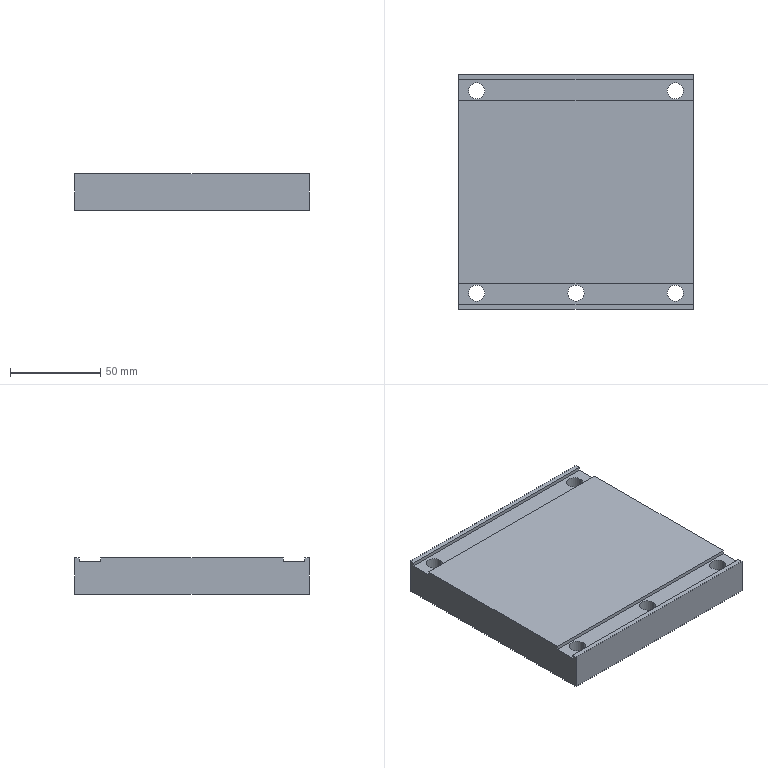Part | STEP file | Head fixing plate | 1 solid | 46 faces | box 130 x 130 x 20 mm | volume 311924 mm3 | cylinder 23 | plane 23 | commonest cylinder face diameters 9 x10 15 x10 3 x3
STEP:
#1=CARTESIAN_POINT('',(62.5,56.,-1.));
#2=VERTEX_POINT('',#1);
#3=CARTESIAN_POINT('',(47.5,56.,-1.));
#4=VERTEX_POINT('',#3);
#5=CARTESIAN_POINT('',(55.,56.,-1.));
#6=DIRECTION('',(0.,0.,-1.));
#7=DIRECTION('',(-1.,0.,0.));
#8=AXIS2_PLACEMENT_3D('',#5,#6,#7);
#9=CIRCLE('',#8,7.5);
#10=EDGE_CURVE('',#2,#4,#9,.T.);
#11=ORIENTED_EDGE('',*,*,#10,.F.);
#12=CARTESIAN_POINT('',(62.5,56.,-10.));
#13=VERTEX_POINT('',#12);
#14=CARTESIAN_POINT('',(62.5,56.,-10.));
#15=DIRECTION('',(0.,0.,-1.));
#16=VECTOR('',#15,1000.);
#17=LINE('',#14,#16);
#18=EDGE_CURVE('',#2,#13,#17,.T.);
#19=ORIENTED_EDGE('',*,*,#18,.T.);
#20=CARTESIAN_POINT('',(47.5,56.,-10.));
#21=VERTEX_POINT('',#20);
#22=CARTESIAN_POINT('',(55.,56.,-10.));
#23=DIRECTION('',(0.,0.,-1.));
#24=DIRECTION('',(-1.,0.,0.));
#25=AXIS2_PLACEMENT_3D('',#22,#23,#24);
#26=CIRCLE('',#25,7.5);
#27=EDGE_CURVE('',#13,#21,#26,.T.);
#28=ORIENTED_EDGE('',*,*,#27,.T.);
#29=CARTESIAN_POINT('',(47.5,56.,-10.));
#30=DIRECTION('',(0.,0.,-1.));
#31=VECTOR('',#30,1000.);
#32=LINE('',#29,#31);
#33=EDGE_CURVE('',#4,#21,#32,.T.);
#34=ORIENTED_EDGE('',*,*,#33,.F.);
#35=EDGE_LOOP('',(#11,#19,#28,#34));
#36=FACE_OUTER_BOUND('',#35,.T.);
#37=CARTESIAN_POINT('',(55.,56.,-10.));
#38=DIRECTION('',(0.,0.,-1.));
#39=DIRECTION('',(-1.,0.,0.));
#40=AXIS2_PLACEMENT_3D('',#37,#38,#39);
#41=CYLINDRICAL_SURFACE('',#40,7.5);
#42=ADVANCED_FACE('',(#36),#41,.F.);
#43=CARTESIAN_POINT('',(50.5,56.,8.));
#44=VERTEX_POINT('',#43);
#45=CARTESIAN_POINT('',(59.5,56.,8.));
#46=VERTEX_POINT('',#45);
#47=CARTESIAN_POINT('',(55.,56.,8.));
#48=DIRECTION('',(0.,0.,1.));
#49=DIRECTION('',(1.,0.,0.));
#50=AXIS2_PLACEMENT_3D('',#47,#48,#49);
#51=CIRCLE('',#50,4.5);
#52=EDGE_CURVE('',#44,#46,#51,.T.);
#53=ORIENTED_EDGE('',*,*,#52,.T.);
#54=CARTESIAN_POINT('',(59.5,56.,-1.));
#55=VERTEX_POINT('',#54);
#56=CARTESIAN_POINT('',(59.5,56.,-10.));
#57=DIRECTION('',(0.,0.,-1.));
#58=VECTOR('',#57,1000.);
#59=LINE('',#56,#58);
#60=EDGE_CURVE('',#46,#55,#59,.T.);
#61=ORIENTED_EDGE('',*,*,#60,.T.);
#62=CARTESIAN_POINT('',(50.5,56.,-1.));
#63=VERTEX_POINT('',#62);
#64=CARTESIAN_POINT('',(55.,56.,-1.));
#65=DIRECTION('',(0.,0.,-1.));
#66=DIRECTION('',(-1.,0.,0.));
#67=AXIS2_PLACEMENT_3D('',#64,#65,#66);
#68=CIRCLE('',#67,4.5);
#69=EDGE_CURVE('',#55,#63,#68,.T.);
#70=ORIENTED_EDGE('',*,*,#69,.T.);
#71=CARTESIAN_POINT('',(50.5,56.,-10.));
#72=DIRECTION('',(0.,0.,-1.));
#73=VECTOR('',#72,1000.);
#74=LINE('',#71,#73);
#75=EDGE_CURVE('',#44,#63,#74,.T.);
#76=ORIENTED_EDGE('',*,*,#75,.F.);
#77=EDGE_LOOP('',(#53,#61,#70,#76));
#78=FACE_OUTER_BOUND('',#77,.T.);
#79=CARTESIAN_POINT('',(55.,56.,-10.));
#80=DIRECTION('',(0.,0.,-1.));
#81=DIRECTION('',(-1.,0.,0.));
#82=AXIS2_PLACEMENT_3D('',#79,#80,#81);
#83=CYLINDRICAL_SURFACE('',#82,4.5);
#84=ADVANCED_FACE('',(#78),#83,.F.);
#85=CARTESIAN_POINT('',(-47.5,56.,-1.));
#86=VERTEX_POINT('',#85);
#87=CARTESIAN_POINT('',(-62.5,56.,-1.));
#88=VERTEX_POINT('',#87);
#89=CARTESIAN_POINT('',(-55.,56.,-1.));
#90=DIRECTION('',(0.,0.,-1.));
#91=DIRECTION('',(-1.,0.,0.));
#92=AXIS2_PLACEMENT_3D('',#89,#90,#91);
#93=CIRCLE('',#92,7.5);
#94=EDGE_CURVE('',#86,#88,#93,.T.);
#95=ORIENTED_EDGE('',*,*,#94,.F.);
#96=CARTESIAN_POINT('',(-47.5,56.,-10.));
#97=VERTEX_POINT('',#96);
#98=CARTESIAN_POINT('',(-47.5,56.,-10.));
#99=DIRECTION('',(0.,0.,-1.));
#100=VECTOR('',#99,1000.);
#101=LINE('',#98,#100);
#102=EDGE_CURVE('',#86,#97,#101,.T.);
#103=ORIENTED_EDGE('',*,*,#102,.T.);
#104=CARTESIAN_POINT('',(-62.5,56.,-10.));
#105=VERTEX_POINT('',#104);
#106=CARTESIAN_POINT('',(-55.,56.,-10.));
#107=DIRECTION('',(0.,0.,-1.));
#108=DIRECTION('',(-1.,0.,0.));
#109=AXIS2_PLACEMENT_3D('',#106,#107,#108);
#110=CIRCLE('',#109,7.5);
#111=EDGE_CURVE('',#97,#105,#110,.T.);
#112=ORIENTED_EDGE('',*,*,#111,.T.);
#113=CARTESIAN_POINT('',(-62.5,56.,-10.));
#114=DIRECTION('',(0.,0.,-1.));
#115=VECTOR('',#114,1000.);
#116=LINE('',#113,#115);
#117=EDGE_CURVE('',#88,#105,#116,.T.);
#118=ORIENTED_EDGE('',*,*,#117,.F.);
#119=EDGE_LOOP('',(#95,#103,#112,#118));
#120=FACE_OUTER_BOUND('',#119,.T.);
#121=CARTESIAN_POINT('',(-55.,56.,-10.));
#122=DIRECTION('',(0.,0.,-1.));
#123=DIRECTION('',(-1.,0.,0.));
#124=AXIS2_PLACEMENT_3D('',#121,#122,#123);
#125=CYLINDRICAL_SURFACE('',#124,7.5);
#126=ADVANCED_FACE('',(#120),#125,.F.);
#127=CARTESIAN_POINT('',(-59.5,56.,8.));
#128=VERTEX_POINT('',#127);
#129=CARTESIAN_POINT('',(-50.5,56.,8.));
#130=VERTEX_POINT('',#129);
#131=CARTESIAN_POINT('',(-55.,56.,8.));
#132=DIRECTION('',(0.,0.,1.));
#133=DIRECTION('',(1.,0.,0.));
#134=AXIS2_PLACEMENT_3D('',#131,#132,#133);
#135=CIRCLE('',#134,4.5);
#136=EDGE_CURVE('',#128,#130,#135,.T.);
#137=ORIENTED_EDGE('',*,*,#136,.T.);
#138=CARTESIAN_POINT('',(-50.5,56.,-1.));
#139=VERTEX_POINT('',#138);
#140=CARTESIAN_POINT('',(-50.5,56.,-10.));
#141=DIRECTION('',(0.,0.,-1.));
#142=VECTOR('',#141,1000.);
#143=LINE('',#140,#142);
#144=EDGE_CURVE('',#130,#139,#143,.T.);
#145=ORIENTED_EDGE('',*,*,#144,.T.);
#146=CARTESIAN_POINT('',(-59.5,56.,-1.));
#147=VERTEX_POINT('',#146);
#148=CARTESIAN_POINT('',(-55.,56.,-1.));
#149=DIRECTION('',(0.,0.,-1.));
#150=DIRECTION('',(-1.,0.,0.));
#151=AXIS2_PLACEMENT_3D('',#148,#149,#150);
#152=CIRCLE('',#151,4.5);
#153=EDGE_CURVE('',#139,#147,#152,.T.);
#154=ORIENTED_EDGE('',*,*,#153,.T.);
#155=CARTESIAN_POINT('',(-59.5,56.,-10.));
#156=DIRECTION('',(0.,0.,-1.));
#157=VECTOR('',#156,1000.);
#158=LINE('',#155,#157);
#159=EDGE_CURVE('',#128,#147,#158,.T.);
#160=ORIENTED_EDGE('',*,*,#159,.F.);
#161=EDGE_LOOP('',(#137,#145,#154,#160));
#162=FACE_OUTER_BOUND('',#161,.T.);
#163=CARTESIAN_POINT('',(-55.,56.,-10.));
#164=DIRECTION('',(0.,0.,-1.));
#165=DIRECTION('',(-1.,0.,0.));
#166=AXIS2_PLACEMENT_3D('',#163,#164,#165);
#167=CYLINDRICAL_SURFACE('',#166,4.5);
#168=ADVANCED_FACE('',(#162),#167,.F.);
#169=CARTESIAN_POINT('',(62.5,-56.,-1.));
#170=VERTEX_POINT('',#169);
#171=CARTESIAN_POINT('',(47.5,-56.,-1.));
#172=VERTEX_POINT('',#171);
#173=CARTESIAN_POINT('',(55.,-56.,-1.));
#174=DIRECTION('',(0.,0.,-1.));
#175=DIRECTION('',(-1.,0.,0.));
#176=AXIS2_PLACEMENT_3D('',#173,#174,#175);
#177=CIRCLE('',#176,7.5);
#178=EDGE_CURVE('',#170,#172,#177,.T.);
#179=ORIENTED_EDGE('',*,*,#178,.F.);
#180=CARTESIAN_POINT('',(62.5,-56.,-10.));
#181=VERTEX_POINT('',#180);
#182=CARTESIAN_POINT('',(62.5,-56.,-10.));
#183=DIRECTION('',(0.,0.,-1.));
#184=VECTOR('',#183,1000.);
#185=LINE('',#182,#184);
#186=EDGE_CURVE('',#170,#181,#185,.T.);
#187=ORIENTED_EDGE('',*,*,#186,.T.);
#188=CARTESIAN_POINT('',(47.5,-56.,-10.));
#189=VERTEX_POINT('',#188);
#190=CARTESIAN_POINT('',(55.,-56.,-10.));
#191=DIRECTION('',(0.,0.,-1.));
#192=DIRECTION('',(-1.,0.,0.));
#193=AXIS2_PLACEMENT_3D('',#190,#191,#192);
#194=CIRCLE('',#193,7.5);
#195=EDGE_CURVE('',#181,#189,#194,.T.);
#196=ORIENTED_EDGE('',*,*,#195,.T.);
#197=CARTESIAN_POINT('',(47.5,-56.,-10.));
#198=DIRECTION('',(0.,0.,-1.));
#199=VECTOR('',#198,1000.);
#200=LINE('',#197,#199);
#201=EDGE_CURVE('',#172,#189,#200,.T.);
#202=ORIENTED_EDGE('',*,*,#201,.F.);
#203=EDGE_LOOP('',(#179,#187,#196,#202));
#204=FACE_OUTER_BOUND('',#203,.T.);
#205=CARTESIAN_POINT('',(55.,-56.,-10.));
#206=DIRECTION('',(0.,0.,-1.));
#207=DIRECTION('',(-1.,0.,0.));
#208=AXIS2_PLACEMENT_3D('',#205,#206,#207);
#209=CYLINDRICAL_SURFACE('',#208,7.5);
#210=ADVANCED_FACE('',(#204),#209,.F.);
#211=CARTESIAN_POINT('',(50.5,-56.,8.));
#212=VERTEX_POINT('',#211);
#213=CARTESIAN_POINT('',(59.5,-56.,8.));
#214=VERTEX_POINT('',#213);
#215=CARTESIAN_POINT('',(55.,-56.,8.));
#216=DIRECTION('',(0.,0.,1.));
#217=DIRECTION('',(1.,0.,0.));
#218=AXIS2_PLACEMENT_3D('',#215,#216,#217);
#219=CIRCLE('',#218,4.5);
#220=EDGE_CURVE('',#212,#214,#219,.T.);
#221=ORIENTED_EDGE('',*,*,#220,.T.);
#222=CARTESIAN_POINT('',(59.5,-56.,-1.));
#223=VERTEX_POINT('',#222);
#224=CARTESIAN_POINT('',(59.5,-56.,-10.));
#225=DIRECTION('',(0.,0.,-1.));
#226=VECTOR('',#225,1000.);
#227=LINE('',#224,#226);
#228=EDGE_CURVE('',#214,#223,#227,.T.);
#229=ORIENTED_EDGE('',*,*,#228,.T.);
#230=CARTESIAN_POINT('',(50.5,-56.,-1.));
#231=VERTEX_POINT('',#230);
#232=CARTESIAN_POINT('',(55.,-56.,-1.));
#233=DIRECTION('',(0.,0.,-1.));
#234=DIRECTION('',(-1.,0.,0.));
#235=AXIS2_PLACEMENT_3D('',#232,#233,#234);
#236=CIRCLE('',#235,4.5);
#237=EDGE_CURVE('',#223,#231,#236,.T.);
#238=ORIENTED_EDGE('',*,*,#237,.T.);
#239=CARTESIAN_POINT('',(50.5,-56.,-10.));
#240=DIRECTION('',(0.,0.,-1.));
#241=VECTOR('',#240,1000.);
#242=LINE('',#239,#241);
#243=EDGE_CURVE('',#212,#231,#242,.T.);
#244=ORIENTED_EDGE('',*,*,#243,.F.);
#245=EDGE_LOOP('',(#221,#229,#238,#244));
#246=FACE_OUTER_BOUND('',#245,.T.);
#247=CARTESIAN_POINT('',(55.,-56.,-10.));
#248=DIRECTION('',(0.,0.,-1.));
#249=DIRECTION('',(-1.,0.,0.));
#250=AXIS2_PLACEMENT_3D('',#247,#248,#249);
#251=CYLINDRICAL_SURFACE('',#250,4.5);
#252=ADVANCED_FACE('',(#246),#251,.F.);
#253=CARTESIAN_POINT('',(7.5,-56.,-1.));
#254=VERTEX_POINT('',#253);
#255=CARTESIAN_POINT('',(-7.5,-56.,-1.));
#256=VERTEX_POINT('',#255);
#257=CARTESIAN_POINT('',(0.,-56.,-1.));
#258=DIRECTION('',(0.,0.,-1.));
#259=DIRECTION('',(-1.,0.,0.));
#260=AXIS2_PLACEMENT_3D('',#257,#258,#259);
#261=CIRCLE('',#260,7.5);
#262=EDGE_CURVE('',#254,#256,#261,.T.);
#263=ORIENTED_EDGE('',*,*,#262,.F.);
#264=CARTESIAN_POINT('',(7.5,-56.,-10.));
#265=VERTEX_POINT('',#264);
#266=CARTESIAN_POINT('',(7.5,-56.,-10.));
#267=DIRECTION('',(0.,0.,-1.));
#268=VECTOR('',#267,1000.);
#269=LINE('',#266,#268);
#270=EDGE_CURVE('',#254,#265,#269,.T.);
#271=ORIENTED_EDGE('',*,*,#270,.T.);
#272=CARTESIAN_POINT('',(-7.5,-56.,-10.));
#273=VERTEX_POINT('',#272);
#274=CARTESIAN_POINT('',(0.,-56.,-10.));
#275=DIRECTION('',(0.,0.,-1.));
#276=DIRECTION('',(-1.,0.,0.));
#277=AXIS2_PLACEMENT_3D('',#274,#275,#276);
#278=CIRCLE('',#277,7.5);
#279=EDGE_CURVE('',#265,#273,#278,.T.);
#280=ORIENTED_EDGE('',*,*,#279,.T.);
#281=CARTESIAN_POINT('',(-7.5,-56.,-10.));
#282=DIRECTION('',(0.,0.,-1.));
#283=VECTOR('',#282,1000.);
#284=LINE('',#281,#283);
#285=EDGE_CURVE('',#256,#273,#284,.T.);
#286=ORIENTED_EDGE('',*,*,#285,.F.);
#287=EDGE_LOOP('',(#263,#271,#280,#286));
#288=FACE_OUTER_BOUND('',#287,.T.);
#289=CARTESIAN_POINT('',(0.,-56.,-10.));
#290=DIRECTION('',(0.,0.,-1.));
#291=DIRECTION('',(-1.,0.,0.));
#292=AXIS2_PLACEMENT_3D('',#289,#290,#291);
#293=CYLINDRICAL_SURFACE('',#292,7.5);
#294=ADVANCED_FACE('',(#288),#293,.F.);
#295=CARTESIAN_POINT('',(-4.5,-56.,8.));
#296=VERTEX_POINT('',#295);
#297=CARTESIAN_POINT('',(4.5,-56.,8.));
#298=VERTEX_POINT('',#297);
#299=CARTESIAN_POINT('',(0.,-56.,8.));
#300=DIRECTION('',(0.,0.,1.));
#301=DIRECTION('',(1.,0.,0.));
#302=AXIS2_PLACEMENT_3D('',#299,#300,#301);
#303=CIRCLE('',#302,4.5);
#304=EDGE_CURVE('',#296,#298,#303,.T.);
#305=ORIENTED_EDGE('',*,*,#304,.T.);
#306=CARTESIAN_POINT('',(4.5,-56.,-1.));
#307=VERTEX_POINT('',#306);
#308=CARTESIAN_POINT('',(4.5,-56.,-10.));
#309=DIRECTION('',(0.,0.,-1.));
#310=VECTOR('',#309,1000.);
#311=LINE('',#308,#310);
#312=EDGE_CURVE('',#298,#307,#311,.T.);
#313=ORIENTED_EDGE('',*,*,#312,.T.);
#314=CARTESIAN_POINT('',(-4.5,-56.,-1.));
#315=VERTEX_POINT('',#314);
#316=CARTESIAN_POINT('',(0.,-56.,-1.));
#317=DIRECTION('',(0.,0.,-1.));
#318=DIRECTION('',(-1.,0.,0.));
#319=AXIS2_PLACEMENT_3D('',#316,#317,#318);
#320=CIRCLE('',#319,4.5);
#321=EDGE_CURVE('',#307,#315,#320,.T.);
#322=ORIENTED_EDGE('',*,*,#321,.T.);
#323=CARTESIAN_POINT('',(-4.5,-56.,-10.));
#324=DIRECTION('',(0.,0.,-1.));
#325=VECTOR('',#324,1000.);
#326=LINE('',#323,#325);
#327=EDGE_CURVE('',#296,#315,#326,.T.);
#328=ORIENTED_EDGE('',*,*,#327,.F.);
#329=EDGE_LOOP('',(#305,#313,#322,#328));
#330=FACE_OUTER_BOUND('',#329,.T.);
#331=CARTESIAN_POINT('',(0.,-56.,-10.));
#332=DIRECTION('',(0.,0.,-1.));
#333=DIRECTION('',(-1.,0.,0.));
#334=AXIS2_PLACEMENT_3D('',#331,#332,#333);
#335=CYLINDRICAL_SURFACE('',#334,4.5);
#336=ADVANCED_FACE('',(#330),#335,.F.);
#337=CARTESIAN_POINT('',(-47.5,-56.,-1.));
#338=VERTEX_POINT('',#337);
#339=CARTESIAN_POINT('',(-62.5,-56.,-1.));
#340=VERTEX_POINT('',#339);
#341=CARTESIAN_POINT('',(-55.,-56.,-1.));
#342=DIRECTION('',(0.,0.,-1.));
#343=DIRECTION('',(-1.,0.,0.));
#344=AXIS2_PLACEMENT_3D('',#341,#342,#343);
#345=CIRCLE('',#344,7.5);
#346=EDGE_CURVE('',#338,#340,#345,.T.);
#347=ORIENTED_EDGE('',*,*,#346,.F.);
#348=CARTESIAN_POINT('',(-47.5,-56.,-10.));
#349=VERTEX_POINT('',#348);
#350=CARTESIAN_POINT('',(-47.5,-56.,-10.));
#351=DIRECTION('',(0.,0.,-1.));
#352=VECTOR('',#351,1000.);
#353=LINE('',#350,#352);
#354=EDGE_CURVE('',#338,#349,#353,.T.);
#355=ORIENTED_EDGE('',*,*,#354,.T.);
#356=CARTESIAN_POINT('',(-62.5,-56.,-10.));
#357=VERTEX_POINT('',#356);
#358=CARTESIAN_POINT('',(-55.,-56.,-10.));
#359=DIRECTION('',(0.,0.,-1.));
#360=DIRECTION('',(-1.,0.,0.));
#361=AXIS2_PLACEMENT_3D('',#358,#359,#360);
#362=CIRCLE('',#361,7.5);
#363=EDGE_CURVE('',#349,#357,#362,.T.);
#364=ORIENTED_EDGE('',*,*,#363,.T.);
#365=CARTESIAN_POINT('',(-62.5,-56.,-10.));
#366=DIRECTION('',(0.,0.,-1.));
#367=VECTOR('',#366,1000.);
#368=LINE('',#365,#367);
#369=EDGE_CURVE('',#340,#357,#368,.T.);
#370=ORIENTED_EDGE('',*,*,#369,.F.);
#371=EDGE_LOOP('',(#347,#355,#364,#370));
#372=FACE_OUTER_BOUND('',#371,.T.);
#373=CARTESIAN_POINT('',(-55.,-56.,-10.));
#374=DIRECTION('',(0.,0.,-1.));
#375=DIRECTION('',(-1.,0.,0.));
#376=AXIS2_PLACEMENT_3D('',#373,#374,#375);
#377=CYLINDRICAL_SURFACE('',#376,7.5);
#378=ADVANCED_FACE('',(#372),#377,.F.);
#379=CARTESIAN_POINT('',(-59.5,-56.,8.));
#380=VERTEX_POINT('',#379);
#381=CARTESIAN_POINT('',(-50.5,-56.,8.));
#382=VERTEX_POINT('',#381);
#383=CARTESIAN_POINT('',(-55.,-56.,8.));
#384=DIRECTION('',(0.,0.,1.));
#385=DIRECTION('',(1.,0.,0.));
#386=AXIS2_PLACEMENT_3D('',#383,#384,#385);
#387=CIRCLE('',#386,4.5);
#388=EDGE_CURVE('',#380,#382,#387,.T.);
#389=ORIENTED_EDGE('',*,*,#388,.T.);
#390=CARTESIAN_POINT('',(-50.5,-56.,-1.));
#391=VERTEX_POINT('',#390);
#392=CARTESIAN_POINT('',(-50.5,-56.,-10.));
#393=DIRECTION('',(0.,0.,-1.));
#394=VECTOR('',#393,1000.);
#395=LINE('',#392,#394);
#396=EDGE_CURVE('',#382,#391,#395,.T.);
#397=ORIENTED_EDGE('',*,*,#396,.T.);
#398=CARTESIAN_POINT('',(-59.5,-56.,-1.));
#399=VERTEX_POINT('',#398);
#400=CARTESIAN_POINT('',(-55.,-56.,-1.));
#401=DIRECTION('',(0.,0.,-1.));
#402=DIRECTION('',(-1.,0.,0.));
#403=AXIS2_PLACEMENT_3D('',#400,#401,#402);
#404=CIRCLE('',#403,4.5);
#405=EDGE_CURVE('',#391,#399,#404,.T.);
#406=ORIENTED_EDGE('',*,*,#405,.T.);
#407=CARTESIAN_POINT('',(-59.5,-56.,-10.));
#408=DIRECTION('',(0.,0.,-1.));
#409=VECTOR('',#408,1000.);
#410=LINE('',#407,#409);
#411=EDGE_CURVE('',#380,#399,#410,.T.);
#412=ORIENTED_EDGE('',*,*,#411,.F.);
#413=EDGE_LOOP('',(#389,#397,#406,#412));
#414=FACE_OUTER_BOUND('',#413,.T.);
#415=CARTESIAN_POINT('',(-55.,-56.,-10.));
#416=DIRECTION('',(0.,0.,-1.));
#417=DIRECTION('',(-1.,0.,0.));
#418=AXIS2_PLACEMENT_3D('',#415,#416,#417);
#419=CYLINDRICAL_SURFACE('',#418,4.5);
#420=ADVANCED_FACE('',(#414),#419,.F.);
#421=CARTESIAN_POINT('',(-39.,5.,-8.));
#422=VERTEX_POINT('',#421);
#423=CARTESIAN_POINT('',(-37.5,6.5,-8.));
#424=VERTEX_POINT('',#423);
#425=CARTESIAN_POINT('',(-37.5,5.,-8.));
#426=DIRECTION('',(0.,0.,-1.));
#427=DIRECTION('',(-1.,0.,0.));
#428=AXIS2_PLACEMENT_3D('',#425,#426,#427);
#429=CIRCLE('',#428,1.5);
#430=EDGE_CURVE('',#422,#424,#429,.T.);
#431=ORIENTED_EDGE('',*,*,#430,.F.);
#432=CARTESIAN_POINT('',(-39.,5.,-10.));
#433=VERTEX_POINT('',#432);
#434=CARTESIAN_POINT('',(-39.,5.,-8.));
#435=DIRECTION('',(0.,0.,-1.));
#436=VECTOR('',#435,1000.);
#437=LINE('',#434,#436);
#438=EDGE_CURVE('',#422,#433,#437,.T.);
#439=ORIENTED_EDGE('',*,*,#438,.T.);
#440=CARTESIAN_POINT('',(-37.5,6.5,-10.));
#441=VERTEX_POINT('',#440);
#442=CARTESIAN_POINT('',(-37.5,5.,-10.));
#443=DIRECTION('',(0.,0.,-1.));
#444=DIRECTION('',(-1.,0.,0.));
#445=AXIS2_PLACEMENT_3D('',#442,#443,#444);
#446=CIRCLE('',#445,1.5);
#447=EDGE_CURVE('',#433,#441,#446,.T.);
#448=ORIENTED_EDGE('',*,*,#447,.T.);
#449=CARTESIAN_POINT('',(-37.5,6.5,-8.));
#450=DIRECTION('',(0.,0.,-1.));
#451=VECTOR('',#450,1000.);
#452=LINE('',#449,#451);
#453=EDGE_CURVE('',#424,#441,#452,.T.);
#454=ORIENTED_EDGE('',*,*,#453,.F.);
#455=EDGE_LOOP('',(#431,#439,#448,#454));
#456=FACE_OUTER_BOUND('',#455,.T.);
#457=CARTESIAN_POINT('',(-37.5,5.,-8.));
#458=DIRECTION('',(0.,0.,-1.));
#459=DIRECTION('',(-1.,0.,0.));
#460=AXIS2_PLACEMENT_3D('',#457,#458,#459);
#461=CYLINDRICAL_SURFACE('',#460,1.5);
#462=ADVANCED_FACE('',(#456),#461,.F.);
#463=CARTESIAN_POINT('',(-65.,-62.5,10.));
#464=VERTEX_POINT('',#463);
#465=CARTESIAN_POINT('',(65.,-62.5,10.));
#466=VERTEX_POINT('',#465);
#467=CARTESIAN_POINT('',(-65.,-62.5,10.));
#468=DIRECTION('',(1.,0.,0.));
#469=VECTOR('',#468,1000.);
#470=LINE('',#467,#469);
#471=EDGE_CURVE('',#464,#466,#470,.T.);
#472=ORIENTED_EDGE('',*,*,#471,.F.);
#473=CARTESIAN_POINT('',(-65.,-65.,10.));
#474=VERTEX_POINT('',#473);
#475=CARTESIAN_POINT('',(-65.,65.,10.));
#476=DIRECTION('',(0.,-1.,0.));
#477=VECTOR('',#476,1000.);
#478=LINE('',#475,#477);
#479=EDGE_CURVE('',#464,#474,#478,.T.);
#480=ORIENTED_EDGE('',*,*,#479,.T.);
#481=CARTESIAN_POINT('',(65.,-65.,10.));
#482=VERTEX_POINT('',#481);
#483=CARTESIAN_POINT('',(-65.,-65.,10.));
#484=DIRECTION('',(1.,0.,0.));
#485=VECTOR('',#484,1000.);
#486=LINE('',#483,#485);
#487=EDGE_CURVE('',#474,#482,#486,.T.);
#488=ORIENTED_EDGE('',*,*,#487,.T.);
#489=CARTESIAN_POINT('',(65.,65.,10.));
#490=DIRECTION('',(0.,1.,0.));
#491=VECTOR('',#490,1000.);
#492=LINE('',#489,#491);
#493=EDGE_CURVE('',#482,#466,#492,.T.);
#494=ORIENTED_EDGE('',*,*,#493,.T.);
#495=EDGE_LOOP('',(#472,#480,#488,#494));
#496=FACE_OUTER_BOUND('',#495,.T.);
#497=CARTESIAN_POINT('',(0.,0.,10.));
#498=DIRECTION('',(0.,0.,1.));
#499=DIRECTION('',(1.,0.,0.));
#500=AXIS2_PLACEMENT_3D('',#497,#498,#499);
#501=PLANE('',#500);
#502=ADVANCED_FACE('',(#496),#501,.T.);
#503=CARTESIAN_POINT('',(65.,62.5,10.));
#504=VERTEX_POINT('',#503);
#505=CARTESIAN_POINT('',(-65.,62.5,10.));
#506=VERTEX_POINT('',#505);
#507=CARTESIAN_POINT('',(-65.,62.5,10.));
#508=DIRECTION('',(-1.,0.,0.));
#509=VECTOR('',#508,1000.);
#510=LINE('',#507,#509);
#511=EDGE_CURVE('',#504,#506,#510,.T.);
#512=ORIENTED_EDGE('',*,*,#511,.F.);
#513=CARTESIAN_POINT('',(65.,65.,10.));
#514=VERTEX_POINT('',#513);
#515=CARTESIAN_POINT('',(65.,65.,10.));
#516=DIRECTION('',(0.,1.,0.));
#517=VECTOR('',#516,1000.);
#518=LINE('',#515,#517);
#519=EDGE_CURVE('',#504,#514,#518,.T.);
#520=ORIENTED_EDGE('',*,*,#519,.T.);
#521=CARTESIAN_POINT('',(-65.,65.,10.));
#522=VERTEX_POINT('',#521);
#523=CARTESIAN_POINT('',(-65.,65.,10.));
#524=DIRECTION('',(-1.,0.,0.));
#525=VECTOR('',#524,1000.);
#526=LINE('',#523,#525);
#527=EDGE_CURVE('',#514,#522,#526,.T.);
#528=ORIENTED_EDGE('',*,*,#527,.T.);
#529=CARTESIAN_POINT('',(-65.,65.,10.));
#530=DIRECTION('',(0.,-1.,0.));
#531=VECTOR('',#530,1000.);
#532=LINE('',#529,#531);
#533=EDGE_CURVE('',#522,#506,#532,.T.);
#534=ORIENTED_EDGE('',*,*,#533,.T.);
#535=EDGE_LOOP('',(#512,#520,#528,#534));
#536=FACE_OUTER_BOUND('',#535,.T.);
#537=CARTESIAN_POINT('',(0.,0.,10.));
#538=DIRECTION('',(0.,0.,1.));
#539=DIRECTION('',(1.,0.,0.));
#540=AXIS2_PLACEMENT_3D('',#537,#538,#539);
#541=PLANE('',#540);
#542=ADVANCED_FACE('',(#536),#541,.T.);
#543=CARTESIAN_POINT('',(65.,-62.5,8.));
#544=VERTEX_POINT('',#543);
#545=CARTESIAN_POINT('',(65.,-50.5,8.));
#546=VERTEX_POINT('',#545);
#547=CARTESIAN_POINT('',(65.,-62.5,8.));
#548=DIRECTION('',(0.,1.,0.));
#549=VECTOR('',#548,1000.);
#550=LINE('',#547,#549);
#551=EDGE_CURVE('',#544,#546,#550,.T.);
#552=ORIENTED_EDGE('',*,*,#551,.F.);
#553=CARTESIAN_POINT('',(65.,-62.5,8.));
#554=DIRECTION('',(0.,0.,1.));
#555=VECTOR('',#554,1000.);
#556=LINE('',#553,#555);
#557=EDGE_CURVE('',#544,#466,#556,.T.);
#558=ORIENTED_EDGE('',*,*,#557,.T.);
#559=ORIENTED_EDGE('',*,*,#493,.F.);
#560=CARTESIAN_POINT('',(65.,-65.,-10.));
#561=VERTEX_POINT('',#560);
#562=CARTESIAN_POINT('',(65.,-65.,10.));
#563=DIRECTION('',(0.,0.,-1.));
#564=VECTOR('',#563,1000.);
#565=LINE('',#562,#564);
#566=EDGE_CURVE('',#482,#561,#565,.T.);
#567=ORIENTED_EDGE('',*,*,#566,.T.);
#568=CARTESIAN_POINT('',(65.,65.,-10.));
#569=VERTEX_POINT('',#568);
#570=CARTESIAN_POINT('',(65.,65.,-10.));
#571=DIRECTION('',(0.,1.,0.));
#572=VECTOR('',#571,1000.);
#573=LINE('',#570,#572);
#574=EDGE_CURVE('',#561,#569,#573,.T.);
#575=ORIENTED_EDGE('',*,*,#574,.T.);
#576=CARTESIAN_POINT('',(65.,65.,10.));
#577=DIRECTION('',(0.,0.,-1.));
#578=VECTOR('',#577,1000.);
#579=LINE('',#576,#578);
#580=EDGE_CURVE('',#514,#569,#579,.T.);
#581=ORIENTED_EDGE('',*,*,#580,.F.);
#582=ORIENTED_EDGE('',*,*,#519,.F.);
#583=CARTESIAN_POINT('',(65.,62.5,8.));
#584=VERTEX_POINT('',#583);
#585=CARTESIAN_POINT('',(65.,62.5,8.));
#586=DIRECTION('',(0.,0.,1.));
#587=VECTOR('',#586,1000.);
#588=LINE('',#585,#587);
#589=EDGE_CURVE('',#584,#504,#588,.T.);
#590=ORIENTED_EDGE('',*,*,#589,.F.);
#591=CARTESIAN_POINT('',(65.,50.5,8.));
#592=VERTEX_POINT('',#591);
#593=CARTESIAN_POINT('',(65.,62.5,8.));
#594=DIRECTION('',(0.,1.,0.));
#595=VECTOR('',#594,1000.);
#596=LINE('',#593,#595);
#597=EDGE_CURVE('',#592,#584,#596,.T.);
#598=ORIENTED_EDGE('',*,*,#597,.F.);
#599=CARTESIAN_POINT('',(65.,50.5,10.));
#600=VERTEX_POINT('',#599);
#601=CARTESIAN_POINT('',(65.,50.5,8.));
#602=DIRECTION('',(0.,0.,1.));
#603=VECTOR('',#602,1000.);
#604=LINE('',#601,#603);
#605=EDGE_CURVE('',#592,#600,#604,.T.);
#606=ORIENTED_EDGE('',*,*,#605,.T.);
#607=CARTESIAN_POINT('',(65.,-50.5,10.));
#608=VERTEX_POINT('',#607);
#609=CARTESIAN_POINT('',(65.,65.,10.));
#610=DIRECTION('',(0.,1.,0.));
#611=VECTOR('',#610,1000.);
#612=LINE('',#609,#611);
#613=EDGE_CURVE('',#608,#600,#612,.T.);
#614=ORIENTED_EDGE('',*,*,#613,.F.);
#615=CARTESIAN_POINT('',(65.,-50.5,8.));
#616=DIRECTION('',(0.,0.,1.));
#617=VECTOR('',#616,1000.);
#618=LINE('',#615,#617);
#619=EDGE_CURVE('',#546,#608,#618,.T.);
#620=ORIENTED_EDGE('',*,*,#619,.F.);
#621=EDGE_LOOP('',(#552,#558,#559,#567,#575,#581,#582,#590,#598,#606,#614,#620));
#622=FACE_OUTER_BOUND('',#621,.T.);
#623=CARTESIAN_POINT('',(65.,65.,10.));
#624=DIRECTION('',(-1.,0.,0.));
#625=DIRECTION('',(0.,-1.,0.));
#626=AXIS2_PLACEMENT_3D('',#623,#624,#625);
#627=PLANE('',#626);
#628=ADVANCED_FACE('',(#622),#627,.F.);
#629=CARTESIAN_POINT('',(37.5,65.,-10.));
#630=VERTEX_POINT('',#629);
#631=CARTESIAN_POINT('',(-65.,65.,-10.));
#632=DIRECTION('',(-1.,0.,0.));
#633=VECTOR('',#632,1000.);
#634=LINE('',#631,#633);
#635=EDGE_CURVE('',#569,#630,#634,.T.);
#636=ORIENTED_EDGE('',*,*,#635,.T.);
#637=CARTESIAN_POINT('',(37.5,65.,-8.));
#638=VERTEX_POINT('',#637);
#639=CARTESIAN_POINT('',(37.5,65.,-8.));
#640=DIRECTION('',(0.,0.,-1.));
#641=VECTOR('',#640,1000.);
#642=LINE('',#639,#641);
#643=EDGE_CURVE('',#638,#630,#642,.T.);
#644=ORIENTED_EDGE('',*,*,#643,.F.);
#645=CARTESIAN_POINT('',(-37.5,65.,-8.));
#646=VERTEX_POINT('',#645);
#647=CARTESIAN_POINT('',(37.5,65.,-8.));
#648=DIRECTION('',(1.,0.,0.));
#649=VECTOR('',#648,1000.);
#650=LINE('',#647,#649);
#651=EDGE_CURVE('',#646,#638,#650,.T.);
#652=ORIENTED_EDGE('',*,*,#651,.F.);
#653=CARTESIAN_POINT('',(-37.5,65.,-10.));
#654=VERTEX_POINT('',#653);
#655=CARTESIAN_POINT('',(-37.5,65.,-8.));
#656=DIRECTION('',(0.,0.,-1.));
#657=VECTOR('',#656,1000.);
#658=LINE('',#655,#657);
#659=EDGE_CURVE('',#646,#654,#658,.T.);
#660=ORIENTED_EDGE('',*,*,#659,.T.);
#661=CARTESIAN_POINT('',(-65.,65.,-10.));
#662=VERTEX_POINT('',#661);
#663=CARTESIAN_POINT('',(-65.,65.,-10.));
#664=DIRECTION('',(-1.,0.,0.));
#665=VECTOR('',#664,1000.);
#666=LINE('',#663,#665);
#667=EDGE_CURVE('',#654,#662,#666,.T.);
#668=ORIENTED_EDGE('',*,*,#667,.T.);
#669=CARTESIAN_POINT('',(-65.,65.,10.));
#670=DIRECTION('',(0.,0.,-1.));
#671=VECTOR('',#670,1000.);
#672=LINE('',#669,#671);
#673=EDGE_CURVE('',#522,#662,#672,.T.);
#674=ORIENTED_EDGE('',*,*,#673,.F.);
#675=ORIENTED_EDGE('',*,*,#527,.F.);
#676=ORIENTED_EDGE('',*,*,#580,.T.);
#677=EDGE_LOOP('',(#636,#644,#652,#660,#668,#674,#675,#676));
#678=FACE_OUTER_BOUND('',#677,.T.);
#679=CARTESIAN_POINT('',(-65.,65.,10.));
#680=DIRECTION('',(0.,-1.,0.));
#681=DIRECTION('',(0.,0.,-1.));
#682=AXIS2_PLACEMENT_3D('',#679,#680,#681);
#683=PLANE('',#682);
#684=ADVANCED_FACE('',(#678),#683,.F.);
#685=ORIENTED_EDGE('',*,*,#479,.F.);
#686=CARTESIAN_POINT('',(-65.,-62.5,8.));
#687=VERTEX_POINT('',#686);
#688=CARTESIAN_POINT('',(-65.,-62.5,8.));
#689=DIRECTION('',(0.,0.,1.));
#690=VECTOR('',#689,1000.);
#691=LINE('',#688,#690);
#692=EDGE_CURVE('',#687,#464,#691,.T.);
#693=ORIENTED_EDGE('',*,*,#692,.F.);
#694=CARTESIAN_POINT('',(-65.,-50.5,8.));
#695=VERTEX_POINT('',#694);
#696=CARTESIAN_POINT('',(-65.,-62.5,8.));
#697=DIRECTION('',(0.,-1.,0.));
#698=VECTOR('',#697,1000.);
#699=LINE('',#696,#698);
#700=EDGE_CURVE('',#695,#687,#699,.T.);
#701=ORIENTED_EDGE('',*,*,#700,.F.);
#702=CARTESIAN_POINT('',(-65.,-50.5,10.));
#703=VERTEX_POINT('',#702);
#704=CARTESIAN_POINT('',(-65.,-50.5,8.));
#705=DIRECTION('',(0.,0.,1.));
#706=VECTOR('',#705,1000.);
#707=LINE('',#704,#706);
#708=EDGE_CURVE('',#695,#703,#707,.T.);
#709=ORIENTED_EDGE('',*,*,#708,.T.);
#710=CARTESIAN_POINT('',(-65.,50.5,10.));
#711=VERTEX_POINT('',#710);
#712=CARTESIAN_POINT('',(-65.,65.,10.));
#713=DIRECTION('',(0.,-1.,0.));
#714=VECTOR('',#713,1000.);
#715=LINE('',#712,#714);
#716=EDGE_CURVE('',#711,#703,#715,.T.);
#717=ORIENTED_EDGE('',*,*,#716,.F.);
#718=CARTESIAN_POINT('',(-65.,50.5,8.));
#719=VERTEX_POINT('',#718);
#720=CARTESIAN_POINT('',(-65.,50.5,8.));
#721=DIRECTION('',(0.,0.,1.));
#722=VECTOR('',#721,1000.);
#723=LINE('',#720,#722);
#724=EDGE_CURVE('',#719,#711,#723,.T.);
#725=ORIENTED_EDGE('',*,*,#724,.F.);
#726=CARTESIAN_POINT('',(-65.,62.5,8.));
#727=VERTEX_POINT('',#726);
#728=CARTESIAN_POINT('',(-65.,62.5,8.));
#729=DIRECTION('',(0.,-1.,0.));
#730=VECTOR('',#729,1000.);
#731=LINE('',#728,#730);
#732=EDGE_CURVE('',#727,#719,#731,.T.);
#733=ORIENTED_EDGE('',*,*,#732,.F.);
#734=CARTESIAN_POINT('',(-65.,62.5,8.));
#735=DIRECTION('',(0.,0.,1.));
#736=VECTOR('',#735,1000.);
#737=LINE('',#734,#736);
#738=EDGE_CURVE('',#727,#506,#737,.T.);
#739=ORIENTED_EDGE('',*,*,#738,.T.);
#740=ORIENTED_EDGE('',*,*,#533,.F.);
#741=ORIENTED_EDGE('',*,*,#673,.T.);
#742=CARTESIAN_POINT('',(-65.,-65.,-10.));
#743=VERTEX_POINT('',#742);
#744=CARTESIAN_POINT('',(-65.,65.,-10.));
#745=DIRECTION('',(0.,-1.,0.));
#746=VECTOR('',#745,1000.);
#747=LINE('',#744,#746);
#748=EDGE_CURVE('',#662,#743,#747,.T.);
#749=ORIENTED_EDGE('',*,*,#748,.T.);
#750=CARTESIAN_POINT('',(-65.,-65.,10.));
#751=DIRECTION('',(0.,0.,-1.));
#752=VECTOR('',#751,1000.);
#753=LINE('',#750,#752);
#754=EDGE_CURVE('',#474,#743,#753,.T.);
#755=ORIENTED_EDGE('',*,*,#754,.F.);
#756=EDGE_LOOP('',(#685,#693,#701,#709,#717,#725,#733,#739,#740,#741,#749,#755));
#757=FACE_OUTER_BOUND('',#756,.T.);
#758=CARTESIAN_POINT('',(-65.,65.,10.));
#759=DIRECTION('',(1.,0.,0.));
#760=DIRECTION('',(0.,1.,0.));
#761=AXIS2_PLACEMENT_3D('',#758,#759,#760);
#762=PLANE('',#761);
#763=ADVANCED_FACE('',(#757),#762,.F.);
#764=CARTESIAN_POINT('',(-65.,-65.,-10.));
#765=DIRECTION('',(1.,0.,0.));
#766=VECTOR('',#765,1000.);
#767=LINE('',#764,#766);
#768=EDGE_CURVE('',#743,#561,#767,.T.);
#769=ORIENTED_EDGE('',*,*,#768,.T.);
#770=ORIENTED_EDGE('',*,*,#566,.F.);
#771=ORIENTED_EDGE('',*,*,#487,.F.);
#772=ORIENTED_EDGE('',*,*,#754,.T.);
#773=EDGE_LOOP('',(#769,#770,#771,#772));
#774=FACE_OUTER_BOUND('',#773,.T.);
#775=CARTESIAN_POINT('',(-65.,-65.,10.));
#776=DIRECTION('',(0.,1.,0.));
#777=DIRECTION('',(-1.,0.,0.));
#778=AXIS2_PLACEMENT_3D('',#775,#776,#777);
#779=PLANE('',#778);
#780=ADVANCED_FACE('',(#774),#779,.F.);
#781=CARTESIAN_POINT('',(-65.,-50.5,10.));
#782=DIRECTION('',(-1.,0.,0.));
#783=VECTOR('',#782,1000.);
#784=LINE('',#781,#783);
#785=EDGE_CURVE('',#608,#703,#784,.T.);
#786=ORIENTED_EDGE('',*,*,#785,.F.);
#787=ORIENTED_EDGE('',*,*,#613,.T.);
#788=CARTESIAN_POINT('',(-65.,50.5,10.));
#789=DIRECTION('',(1.,0.,0.));
#790=VECTOR('',#789,1000.);
#791=LINE('',#788,#790);
#792=EDGE_CURVE('',#711,#600,#791,.T.);
#793=ORIENTED_EDGE('',*,*,#792,.F.);
#794=ORIENTED_EDGE('',*,*,#716,.T.);
#795=EDGE_LOOP('',(#786,#787,#793,#794));
#796=FACE_OUTER_BOUND('',#795,.T.);
#797=CARTESIAN_POINT('',(0.,0.,10.));
#798=DIRECTION('',(0.,0.,1.));
#799=DIRECTION('',(1.,0.,0.));
#800=AXIS2_PLACEMENT_3D('',#797,#798,#799);
#801=PLANE('',#800);
#802=ADVANCED_FACE('',(#796),#801,.T.);
#803=CARTESIAN_POINT('',(55.,56.,-10.));
#804=DIRECTION('',(0.,0.,-1.));
#805=DIRECTION('',(-1.,0.,0.));
#806=AXIS2_PLACEMENT_3D('',#803,#804,#805);
#807=CIRCLE('',#806,7.5);
#808=EDGE_CURVE('',#21,#13,#807,.T.);
#809=ORIENTED_EDGE('',*,*,#808,.F.);
#810=ORIENTED_EDGE('',*,*,#27,.F.);
#811=EDGE_LOOP('',(#809,#810));
#812=FACE_BOUND('',#811,.T.);
#813=CARTESIAN_POINT('',(-55.,56.,-10.));
#814=DIRECTION('',(0.,0.,-1.));
#815=DIRECTION('',(-1.,0.,0.));
#816=AXIS2_PLACEMENT_3D('',#813,#814,#815);
#817=CIRCLE('',#816,7.5);
#818=EDGE_CURVE('',#105,#97,#817,.T.);
#819=ORIENTED_EDGE('',*,*,#818,.F.);
#820=ORIENTED_EDGE('',*,*,#111,.F.);
#821=EDGE_LOOP('',(#819,#820));
#822=FACE_BOUND('',#821,.T.);
#823=CARTESIAN_POINT('',(55.,-56.,-10.));
#824=DIRECTION('',(0.,0.,-1.));
#825=DIRECTION('',(-1.,0.,0.));
#826=AXIS2_PLACEMENT_3D('',#823,#824,#825);
#827=CIRCLE('',#826,7.5);
#828=EDGE_CURVE('',#189,#181,#827,.T.);
#829=ORIENTED_EDGE('',*,*,#828,.F.);
#830=ORIENTED_EDGE('',*,*,#195,.F.);
#831=EDGE_LOOP('',(#829,#830));
#832=FACE_BOUND('',#831,.T.);
#833=CARTESIAN_POINT('',(0.,-56.,-10.));
#834=DIRECTION('',(0.,0.,-1.));
#835=DIRECTION('',(-1.,0.,0.));
#836=AXIS2_PLACEMENT_3D('',#833,#834,#835);
#837=CIRCLE('',#836,7.5);
#838=EDGE_CURVE('',#273,#265,#837,.T.);
#839=ORIENTED_EDGE('',*,*,#838,.F.);
#840=ORIENTED_EDGE('',*,*,#279,.F.);
#841=EDGE_LOOP('',(#839,#840));
#842=FACE_BOUND('',#841,.T.);
#843=CARTESIAN_POINT('',(-55.,-56.,-10.));
#844=DIRECTION('',(0.,0.,-1.));
#845=DIRECTION('',(-1.,0.,0.));
#846=AXIS2_PLACEMENT_3D('',#843,#844,#845);
#847=CIRCLE('',#846,7.5);
#848=EDGE_CURVE('',#357,#349,#847,.T.);
#849=ORIENTED_EDGE('',*,*,#848,.F.);
#850=ORIENTED_EDGE('',*,*,#363,.F.);
#851=EDGE_LOOP('',(#849,#850));
#852=FACE_BOUND('',#851,.T.);
#853=CARTESIAN_POINT('',(-37.5,65.,-10.));
#854=DIRECTION('',(0.,1.,0.));
#855=VECTOR('',#854,1000.);
#856=LINE('',#853,#855);
#857=EDGE_CURVE('',#441,#654,#856,.T.);
#858=ORIENTED_EDGE('',*,*,#857,.F.);
#859=ORIENTED_EDGE('',*,*,#447,.F.);
#860=CARTESIAN_POINT('',(-36.,5.,-10.));
#861=VERTEX_POINT('',#860);
#862=CARTESIAN_POINT('',(-37.5,5.,-10.));
#863=DIRECTION('',(0.,0.,-1.));
#864=DIRECTION('',(-1.,0.,0.));
#865=AXIS2_PLACEMENT_3D('',#862,#863,#864);
#866=CIRCLE('',#865,1.5);
#867=EDGE_CURVE('',#861,#433,#866,.T.);
#868=ORIENTED_EDGE('',*,*,#867,.F.);
#869=CARTESIAN_POINT('',(36.,5.,-10.));
#870=VERTEX_POINT('',#869);
#871=CARTESIAN_POINT('',(37.5,5.,-10.));
#872=DIRECTION('',(-1.,0.,0.));
#873=VECTOR('',#872,1000.);
#874=LINE('',#871,#873);
#875=EDGE_CURVE('',#870,#861,#874,.T.);
#876=ORIENTED_EDGE('',*,*,#875,.F.);
#877=CARTESIAN_POINT('',(37.5,6.5,-10.));
#878=VERTEX_POINT('',#877);
#879=CARTESIAN_POINT('',(37.5,5.,-10.));
#880=DIRECTION('',(0.,0.,-1.));
#881=DIRECTION('',(-1.,0.,0.));
#882=AXIS2_PLACEMENT_3D('',#879,#880,#881);
#883=CIRCLE('',#882,1.5);
#884=EDGE_CURVE('',#878,#870,#883,.T.);
#885=ORIENTED_EDGE('',*,*,#884,.F.);
#886=CARTESIAN_POINT('',(37.5,65.,-10.));
#887=DIRECTION('',(0.,-1.,0.));
#888=VECTOR('',#887,1000.);
#889=LINE('',#886,#888);
#890=EDGE_CURVE('',#630,#878,#889,.T.);
#891=ORIENTED_EDGE('',*,*,#890,.F.);
#892=ORIENTED_EDGE('',*,*,#635,.F.);
#893=ORIENTED_EDGE('',*,*,#574,.F.);
#894=ORIENTED_EDGE('',*,*,#768,.F.);
#895=ORIENTED_EDGE('',*,*,#748,.F.);
#896=ORIENTED_EDGE('',*,*,#667,.F.);
#897=EDGE_LOOP('',(#858,#859,#868,#876,#885,#891,#892,#893,#894,#895,#896));
#898=FACE_OUTER_BOUND('',#897,.T.);
#899=CARTESIAN_POINT('',(0.,0.,-10.));
#900=DIRECTION('',(0.,0.,1.));
#901=DIRECTION('',(1.,0.,0.));
#902=AXIS2_PLACEMENT_3D('',#899,#900,#901);
#903=PLANE('',#902);
#904=ADVANCED_FACE('',(#812,#822,#832,#842,#852,#898),#903,.F.);
#905=ORIENTED_EDGE('',*,*,#890,.T.);
#906=CARTESIAN_POINT('',(37.5,6.5,-8.));
#907=VERTEX_POINT('',#906);
#908=CARTESIAN_POINT('',(37.5,6.5,-8.));
#909=DIRECTION('',(0.,0.,1.));
#910=VECTOR('',#909,1000.);
#911=LINE('',#908,#910);
#912=EDGE_CURVE('',#878,#907,#911,.T.);
#913=ORIENTED_EDGE('',*,*,#912,.T.);
#914=CARTESIAN_POINT('',(37.5,65.,-8.));
#915=DIRECTION('',(0.,-1.,0.));
#916=VECTOR('',#915,1000.);
#917=LINE('',#914,#916);
#918=EDGE_CURVE('',#638,#907,#917,.T.);
#919=ORIENTED_EDGE('',*,*,#918,.F.);
#920=ORIENTED_EDGE('',*,*,#643,.T.);
#921=EDGE_LOOP('',(#905,#913,#919,#920));
#922=FACE_OUTER_BOUND('',#921,.T.);
#923=CARTESIAN_POINT('',(37.5,65.,-8.));
#924=DIRECTION('',(1.,0.,0.));
#925=DIRECTION('',(0.,1.,0.));
#926=AXIS2_PLACEMENT_3D('',#923,#924,#925);
#927=PLANE('',#926);
#928=ADVANCED_FACE('',(#922),#927,.F.);
#929=CARTESIAN_POINT('',(-37.5,65.,-8.));
#930=DIRECTION('',(0.,1.,0.));
#931=VECTOR('',#930,1000.);
#932=LINE('',#929,#931);
#933=EDGE_CURVE('',#424,#646,#932,.T.);
#934=ORIENTED_EDGE('',*,*,#933,.F.);
#935=ORIENTED_EDGE('',*,*,#453,.T.);
#936=ORIENTED_EDGE('',*,*,#857,.T.);
#937=ORIENTED_EDGE('',*,*,#659,.F.);
#938=EDGE_LOOP('',(#934,#935,#936,#937));
#939=FACE_OUTER_BOUND('',#938,.T.);
#940=CARTESIAN_POINT('',(-37.5,65.,-8.));
#941=DIRECTION('',(-1.,0.,0.));
#942=DIRECTION('',(0.,-1.,0.));
#943=AXIS2_PLACEMENT_3D('',#940,#941,#942);
#944=PLANE('',#943);
#945=ADVANCED_FACE('',(#939),#944,.F.);
#946=ORIENTED_EDGE('',*,*,#875,.T.);
#947=CARTESIAN_POINT('',(-36.,5.,-8.));
#948=VERTEX_POINT('',#947);
#949=CARTESIAN_POINT('',(-36.,5.,-8.));
#950=DIRECTION('',(0.,0.,1.));
#951=VECTOR('',#950,1000.);
#952=LINE('',#949,#951);
#953=EDGE_CURVE('',#861,#948,#952,.T.);
#954=ORIENTED_EDGE('',*,*,#953,.T.);
#955=CARTESIAN_POINT('',(36.,5.,-8.));
#956=VERTEX_POINT('',#955);
#957=CARTESIAN_POINT('',(37.5,5.,-8.));
#958=DIRECTION('',(-1.,0.,0.));
#959=VECTOR('',#958,1000.);
#960=LINE('',#957,#959);
#961=EDGE_CURVE('',#956,#948,#960,.T.);
#962=ORIENTED_EDGE('',*,*,#961,.F.);
#963=CARTESIAN_POINT('',(36.,5.,-8.));
#964=DIRECTION('',(0.,0.,-1.));
#965=VECTOR('',#964,1000.);
#966=LINE('',#963,#965);
#967=EDGE_CURVE('',#956,#870,#966,.T.);
#968=ORIENTED_EDGE('',*,*,#967,.T.);
#969=EDGE_LOOP('',(#946,#954,#962,#968));
#970=FACE_OUTER_BOUND('',#969,.T.);
#971=CARTESIAN_POINT('',(37.5,5.,-8.));
#972=DIRECTION('',(0.,-1.,0.));
#973=DIRECTION('',(1.,0.,0.));
#974=AXIS2_PLACEMENT_3D('',#971,#972,#973);
#975=PLANE('',#974);
#976=ADVANCED_FACE('',(#970),#975,.F.);
#977=CARTESIAN_POINT('',(-37.5,5.,-8.));
#978=DIRECTION('',(0.,0.,-1.));
#979=DIRECTION('',(-1.,0.,0.));
#980=AXIS2_PLACEMENT_3D('',#977,#978,#979);
#981=CIRCLE('',#980,1.5);
#982=EDGE_CURVE('',#948,#422,#981,.T.);
#983=ORIENTED_EDGE('',*,*,#982,.T.);
#984=ORIENTED_EDGE('',*,*,#430,.T.);
#985=ORIENTED_EDGE('',*,*,#933,.T.);
#986=ORIENTED_EDGE('',*,*,#651,.T.);
#987=ORIENTED_EDGE('',*,*,#918,.T.);
#988=CARTESIAN_POINT('',(37.5,5.,-8.));
#989=DIRECTION('',(0.,0.,-1.));
#990=DIRECTION('',(-1.,0.,0.));
#991=AXIS2_PLACEMENT_3D('',#988,#989,#990);
#992=CIRCLE('',#991,1.5);
#993=EDGE_CURVE('',#907,#956,#992,.T.);
#994=ORIENTED_EDGE('',*,*,#993,.T.);
#995=ORIENTED_EDGE('',*,*,#961,.T.);
#996=EDGE_LOOP('',(#983,#984,#985,#986,#987,#994,#995));
#997=FACE_OUTER_BOUND('',#996,.T.);
#998=CARTESIAN_POINT('',(0.,0.,-8.));
#999=DIRECTION('',(0.,0.,-1.));
#1000=DIRECTION('',(-1.,0.,0.));
#1001=AXIS2_PLACEMENT_3D('',#998,#999,#1000);
#1002=PLANE('',#1001);
#1003=ADVANCED_FACE('',(#997),#1002,.T.);
#1004=ORIENTED_EDGE('',*,*,#884,.T.);
#1005=ORIENTED_EDGE('',*,*,#967,.F.);
#1006=ORIENTED_EDGE('',*,*,#993,.F.);
#1007=ORIENTED_EDGE('',*,*,#912,.F.);
#1008=EDGE_LOOP('',(#1004,#1005,#1006,#1007));
#1009=FACE_OUTER_BOUND('',#1008,.T.);
#1010=CARTESIAN_POINT('',(37.5,5.,-8.));
#1011=DIRECTION('',(0.,0.,-1.));
#1012=DIRECTION('',(-1.,0.,0.));
#1013=AXIS2_PLACEMENT_3D('',#1010,#1011,#1012);
#1014=CYLINDRICAL_SURFACE('',#1013,1.5);
#1015=ADVANCED_FACE('',(#1009),#1014,.F.);
#1016=ORIENTED_EDGE('',*,*,#438,.F.);
#1017=ORIENTED_EDGE('',*,*,#982,.F.);
#1018=ORIENTED_EDGE('',*,*,#953,.F.);
#1019=ORIENTED_EDGE('',*,*,#867,.T.);
#1020=EDGE_LOOP('',(#1016,#1017,#1018,#1019));
#1021=FACE_OUTER_BOUND('',#1020,.T.);
#1022=CARTESIAN_POINT('',(-37.5,5.,-8.));
#1023=DIRECTION('',(0.,0.,-1.));
#1024=DIRECTION('',(-1.,0.,0.));
#1025=AXIS2_PLACEMENT_3D('',#1022,#1023,#1024);
#1026=CYLINDRICAL_SURFACE('',#1025,1.5);
#1027=ADVANCED_FACE('',(#1021),#1026,.F.);
#1028=ORIENTED_EDGE('',*,*,#511,.T.);
#1029=ORIENTED_EDGE('',*,*,#738,.F.);
#1030=CARTESIAN_POINT('',(-65.,62.5,8.));
#1031=DIRECTION('',(-1.,0.,0.));
#1032=VECTOR('',#1031,1000.);
#1033=LINE('',#1030,#1032);
#1034=EDGE_CURVE('',#584,#727,#1033,.T.);
#1035=ORIENTED_EDGE('',*,*,#1034,.F.);
#1036=ORIENTED_EDGE('',*,*,#589,.T.);
#1037=EDGE_LOOP('',(#1028,#1029,#1035,#1036));
#1038=FACE_OUTER_BOUND('',#1037,.T.);
#1039=CARTESIAN_POINT('',(-65.,62.5,8.));
#1040=DIRECTION('',(0.,1.,0.));
#1041=DIRECTION('',(0.,0.,1.));
#1042=AXIS2_PLACEMENT_3D('',#1039,#1040,#1041);
#1043=PLANE('',#1042);
#1044=ADVANCED_FACE('',(#1038),#1043,.F.);
#1045=ORIENTED_EDGE('',*,*,#792,.T.);
#1046=ORIENTED_EDGE('',*,*,#605,.F.);
#1047=CARTESIAN_POINT('',(-65.,50.5,8.));
#1048=DIRECTION('',(1.,0.,0.));
#1049=VECTOR('',#1048,1000.);
#1050=LINE('',#1047,#1049);
#1051=EDGE_CURVE('',#719,#592,#1050,.T.);
#1052=ORIENTED_EDGE('',*,*,#1051,.F.);
#1053=ORIENTED_EDGE('',*,*,#724,.T.);
#1054=EDGE_LOOP('',(#1045,#1046,#1052,#1053));
#1055=FACE_OUTER_BOUND('',#1054,.T.);
#1056=CARTESIAN_POINT('',(-65.,50.5,8.));
#1057=DIRECTION('',(0.,-1.,0.));
#1058=DIRECTION('',(0.,0.,-1.));
#1059=AXIS2_PLACEMENT_3D('',#1056,#1057,#1058);
#1060=PLANE('',#1059);
#1061=ADVANCED_FACE('',(#1055),#1060,.F.);
#1062=ORIENTED_EDGE('',*,*,#52,.F.);
#1063=CARTESIAN_POINT('',(55.,56.,8.));
#1064=DIRECTION('',(0.,0.,1.));
#1065=DIRECTION('',(1.,0.,0.));
#1066=AXIS2_PLACEMENT_3D('',#1063,#1064,#1065);
#1067=CIRCLE('',#1066,4.5);
#1068=EDGE_CURVE('',#46,#44,#1067,.T.);
#1069=ORIENTED_EDGE('',*,*,#1068,.F.);
#1070=EDGE_LOOP('',(#1062,#1069));
#1071=FACE_BOUND('',#1070,.T.);
#1072=ORIENTED_EDGE('',*,*,#136,.F.);
#1073=CARTESIAN_POINT('',(-55.,56.,8.));
#1074=DIRECTION('',(0.,0.,1.));
#1075=DIRECTION('',(1.,0.,0.));
#1076=AXIS2_PLACEMENT_3D('',#1073,#1074,#1075);
#1077=CIRCLE('',#1076,4.5);
#1078=EDGE_CURVE('',#130,#128,#1077,.T.);
#1079=ORIENTED_EDGE('',*,*,#1078,.F.);
#1080=EDGE_LOOP('',(#1072,#1079));
#1081=FACE_BOUND('',#1080,.T.);
#1082=ORIENTED_EDGE('',*,*,#732,.T.);
#1083=ORIENTED_EDGE('',*,*,#1051,.T.);
#1084=ORIENTED_EDGE('',*,*,#597,.T.);
#1085=ORIENTED_EDGE('',*,*,#1034,.T.);
#1086=EDGE_LOOP('',(#1082,#1083,#1084,#1085));
#1087=FACE_OUTER_BOUND('',#1086,.T.);
#1088=CARTESIAN_POINT('',(0.,0.,8.));
#1089=DIRECTION('',(0.,0.,1.));
#1090=DIRECTION('',(1.,0.,0.));
#1091=AXIS2_PLACEMENT_3D('',#1088,#1089,#1090);
#1092=PLANE('',#1091);
#1093=ADVANCED_FACE('',(#1071,#1081,#1087),#1092,.T.);
#1094=ORIENTED_EDGE('',*,*,#471,.T.);
#1095=ORIENTED_EDGE('',*,*,#557,.F.);
#1096=CARTESIAN_POINT('',(-65.,-62.5,8.));
#1097=DIRECTION('',(1.,0.,0.));
#1098=VECTOR('',#1097,1000.);
#1099=LINE('',#1096,#1098);
#1100=EDGE_CURVE('',#687,#544,#1099,.T.);
#1101=ORIENTED_EDGE('',*,*,#1100,.F.);
#1102=ORIENTED_EDGE('',*,*,#692,.T.);
#1103=EDGE_LOOP('',(#1094,#1095,#1101,#1102));
#1104=FACE_OUTER_BOUND('',#1103,.T.);
#1105=CARTESIAN_POINT('',(-65.,-62.5,8.));
#1106=DIRECTION('',(0.,-1.,0.));
#1107=DIRECTION('',(0.,0.,-1.));
#1108=AXIS2_PLACEMENT_3D('',#1105,#1106,#1107);
#1109=PLANE('',#1108);
#1110=ADVANCED_FACE('',(#1104),#1109,.F.);
#1111=ORIENTED_EDGE('',*,*,#785,.T.);
#1112=ORIENTED_EDGE('',*,*,#708,.F.);
#1113=CARTESIAN_POINT('',(-65.,-50.5,8.));
#1114=DIRECTION('',(-1.,0.,0.));
#1115=VECTOR('',#1114,1000.);
#1116=LINE('',#1113,#1115);
#1117=EDGE_CURVE('',#546,#695,#1116,.T.);
#1118=ORIENTED_EDGE('',*,*,#1117,.F.);
#1119=ORIENTED_EDGE('',*,*,#619,.T.);
#1120=EDGE_LOOP('',(#1111,#1112,#1118,#1119));
#1121=FACE_OUTER_BOUND('',#1120,.T.);
#1122=CARTESIAN_POINT('',(-65.,-50.5,8.));
#1123=DIRECTION('',(0.,1.,0.));
#1124=DIRECTION('',(0.,0.,1.));
#1125=AXIS2_PLACEMENT_3D('',#1122,#1123,#1124);
#1126=PLANE('',#1125);
#1127=ADVANCED_FACE('',(#1121),#1126,.F.);
#1128=ORIENTED_EDGE('',*,*,#220,.F.);
#1129=CARTESIAN_POINT('',(55.,-56.,8.));
#1130=DIRECTION('',(0.,0.,1.));
#1131=DIRECTION('',(1.,0.,0.));
#1132=AXIS2_PLACEMENT_3D('',#1129,#1130,#1131);
#1133=CIRCLE('',#1132,4.5);
#1134=EDGE_CURVE('',#214,#212,#1133,.T.);
#1135=ORIENTED_EDGE('',*,*,#1134,.F.);
#1136=EDGE_LOOP('',(#1128,#1135));
#1137=FACE_BOUND('',#1136,.T.);
#1138=ORIENTED_EDGE('',*,*,#304,.F.);
#1139=CARTESIAN_POINT('',(0.,-56.,8.));
#1140=DIRECTION('',(0.,0.,1.));
#1141=DIRECTION('',(1.,0.,0.));
#1142=AXIS2_PLACEMENT_3D('',#1139,#1140,#1141);
#1143=CIRCLE('',#1142,4.5);
#1144=EDGE_CURVE('',#298,#296,#1143,.T.);
#1145=ORIENTED_EDGE('',*,*,#1144,.F.);
#1146=EDGE_LOOP('',(#1138,#1145));
#1147=FACE_BOUND('',#1146,.T.);
#1148=ORIENTED_EDGE('',*,*,#388,.F.);
#1149=CARTESIAN_POINT('',(-55.,-56.,8.));
#1150=DIRECTION('',(0.,0.,1.));
#1151=DIRECTION('',(1.,0.,0.));
#1152=AXIS2_PLACEMENT_3D('',#1149,#1150,#1151);
#1153=CIRCLE('',#1152,4.5);
#1154=EDGE_CURVE('',#382,#380,#1153,.T.);
#1155=ORIENTED_EDGE('',*,*,#1154,.F.);
#1156=EDGE_LOOP('',(#1148,#1155));
#1157=FACE_BOUND('',#1156,.T.);
#1158=ORIENTED_EDGE('',*,*,#1100,.T.);
#1159=ORIENTED_EDGE('',*,*,#551,.T.);
#1160=ORIENTED_EDGE('',*,*,#1117,.T.);
#1161=ORIENTED_EDGE('',*,*,#700,.T.);
#1162=EDGE_LOOP('',(#1158,#1159,#1160,#1161));
#1163=FACE_OUTER_BOUND('',#1162,.T.);
#1164=CARTESIAN_POINT('',(0.,0.,8.));
#1165=DIRECTION('',(0.,0.,1.));
#1166=DIRECTION('',(1.,0.,0.));
#1167=AXIS2_PLACEMENT_3D('',#1164,#1165,#1166);
#1168=PLANE('',#1167);
#1169=ADVANCED_FACE('',(#1137,#1147,#1157,#1163),#1168,.T.);
#1170=ORIENTED_EDGE('',*,*,#396,.F.);
#1171=ORIENTED_EDGE('',*,*,#1154,.T.);
#1172=ORIENTED_EDGE('',*,*,#411,.T.);
#1173=CARTESIAN_POINT('',(-55.,-56.,-1.));
#1174=DIRECTION('',(0.,0.,-1.));
#1175=DIRECTION('',(-1.,0.,0.));
#1176=AXIS2_PLACEMENT_3D('',#1173,#1174,#1175);
#1177=CIRCLE('',#1176,4.5);
#1178=EDGE_CURVE('',#399,#391,#1177,.T.);
#1179=ORIENTED_EDGE('',*,*,#1178,.T.);
#1180=EDGE_LOOP('',(#1170,#1171,#1172,#1179));
#1181=FACE_OUTER_BOUND('',#1180,.T.);
#1182=CARTESIAN_POINT('',(-55.,-56.,-10.));
#1183=DIRECTION('',(0.,0.,-1.));
#1184=DIRECTION('',(-1.,0.,0.));
#1185=AXIS2_PLACEMENT_3D('',#1182,#1183,#1184);
#1186=CYLINDRICAL_SURFACE('',#1185,4.5);
#1187=ADVANCED_FACE('',(#1181),#1186,.F.);
#1188=ORIENTED_EDGE('',*,*,#1178,.F.);
#1189=ORIENTED_EDGE('',*,*,#405,.F.);
#1190=EDGE_LOOP('',(#1188,#1189));
#1191=FACE_BOUND('',#1190,.T.);
#1192=CARTESIAN_POINT('',(-55.,-56.,-1.));
#1193=DIRECTION('',(0.,0.,-1.));
#1194=DIRECTION('',(-1.,0.,0.));
#1195=AXIS2_PLACEMENT_3D('',#1192,#1193,#1194);
#1196=CIRCLE('',#1195,7.5);
#1197=EDGE_CURVE('',#340,#338,#1196,.T.);
#1198=ORIENTED_EDGE('',*,*,#1197,.T.);
#1199=ORIENTED_EDGE('',*,*,#346,.T.);
#1200=EDGE_LOOP('',(#1198,#1199));
#1201=FACE_OUTER_BOUND('',#1200,.T.);
#1202=CARTESIAN_POINT('',(-50.5,-56.,-1.));
#1203=DIRECTION('',(0.,0.,1.));
#1204=DIRECTION('',(1.,0.,0.));
#1205=AXIS2_PLACEMENT_3D('',#1202,#1203,#1204);
#1206=PLANE('',#1205);
#1207=ADVANCED_FACE('',(#1191,#1201),#1206,.F.);
#1208=ORIENTED_EDGE('',*,*,#354,.F.);
#1209=ORIENTED_EDGE('',*,*,#1197,.F.);
#1210=ORIENTED_EDGE('',*,*,#369,.T.);
#1211=ORIENTED_EDGE('',*,*,#848,.T.);
#1212=EDGE_LOOP('',(#1208,#1209,#1210,#1211));
#1213=FACE_OUTER_BOUND('',#1212,.T.);
#1214=CARTESIAN_POINT('',(-55.,-56.,-10.));
#1215=DIRECTION('',(0.,0.,-1.));
#1216=DIRECTION('',(-1.,0.,0.));
#1217=AXIS2_PLACEMENT_3D('',#1214,#1215,#1216);
#1218=CYLINDRICAL_SURFACE('',#1217,7.5);
#1219=ADVANCED_FACE('',(#1213),#1218,.F.);
#1220=ORIENTED_EDGE('',*,*,#312,.F.);
#1221=ORIENTED_EDGE('',*,*,#1144,.T.);
#1222=ORIENTED_EDGE('',*,*,#327,.T.);
#1223=CARTESIAN_POINT('',(0.,-56.,-1.));
#1224=DIRECTION('',(0.,0.,-1.));
#1225=DIRECTION('',(-1.,0.,0.));
#1226=AXIS2_PLACEMENT_3D('',#1223,#1224,#1225);
#1227=CIRCLE('',#1226,4.5);
#1228=EDGE_CURVE('',#315,#307,#1227,.T.);
#1229=ORIENTED_EDGE('',*,*,#1228,.T.);
#1230=EDGE_LOOP('',(#1220,#1221,#1222,#1229));
#1231=FACE_OUTER_BOUND('',#1230,.T.);
#1232=CARTESIAN_POINT('',(0.,-56.,-10.));
#1233=DIRECTION('',(0.,0.,-1.));
#1234=DIRECTION('',(-1.,0.,0.));
#1235=AXIS2_PLACEMENT_3D('',#1232,#1233,#1234);
#1236=CYLINDRICAL_SURFACE('',#1235,4.5);
#1237=ADVANCED_FACE('',(#1231),#1236,.F.);
#1238=ORIENTED_EDGE('',*,*,#1228,.F.);
#1239=ORIENTED_EDGE('',*,*,#321,.F.);
#1240=EDGE_LOOP('',(#1238,#1239));
#1241=FACE_BOUND('',#1240,.T.);
#1242=CARTESIAN_POINT('',(0.,-56.,-1.));
#1243=DIRECTION('',(0.,0.,-1.));
#1244=DIRECTION('',(-1.,0.,0.));
#1245=AXIS2_PLACEMENT_3D('',#1242,#1243,#1244);
#1246=CIRCLE('',#1245,7.5);
#1247=EDGE_CURVE('',#256,#254,#1246,.T.);
#1248=ORIENTED_EDGE('',*,*,#1247,.T.);
#1249=ORIENTED_EDGE('',*,*,#262,.T.);
#1250=EDGE_LOOP('',(#1248,#1249));
#1251=FACE_OUTER_BOUND('',#1250,.T.);
#1252=CARTESIAN_POINT('',(4.5,-56.,-1.));
#1253=DIRECTION('',(0.,0.,1.));
#1254=DIRECTION('',(1.,0.,0.));
#1255=AXIS2_PLACEMENT_3D('',#1252,#1253,#1254);
#1256=PLANE('',#1255);
#1257=ADVANCED_FACE('',(#1241,#1251),#1256,.F.);
#1258=ORIENTED_EDGE('',*,*,#270,.F.);
#1259=ORIENTED_EDGE('',*,*,#1247,.F.);
#1260=ORIENTED_EDGE('',*,*,#285,.T.);
#1261=ORIENTED_EDGE('',*,*,#838,.T.);
#1262=EDGE_LOOP('',(#1258,#1259,#1260,#1261));
#1263=FACE_OUTER_BOUND('',#1262,.T.);
#1264=CARTESIAN_POINT('',(0.,-56.,-10.));
#1265=DIRECTION('',(0.,0.,-1.));
#1266=DIRECTION('',(-1.,0.,0.));
#1267=AXIS2_PLACEMENT_3D('',#1264,#1265,#1266);
#1268=CYLINDRICAL_SURFACE('',#1267,7.5);
#1269=ADVANCED_FACE('',(#1263),#1268,.F.);
#1270=ORIENTED_EDGE('',*,*,#228,.F.);
#1271=ORIENTED_EDGE('',*,*,#1134,.T.);
#1272=ORIENTED_EDGE('',*,*,#243,.T.);
#1273=CARTESIAN_POINT('',(55.,-56.,-1.));
#1274=DIRECTION('',(0.,0.,-1.));
#1275=DIRECTION('',(-1.,0.,0.));
#1276=AXIS2_PLACEMENT_3D('',#1273,#1274,#1275);
#1277=CIRCLE('',#1276,4.5);
#1278=EDGE_CURVE('',#231,#223,#1277,.T.);
#1279=ORIENTED_EDGE('',*,*,#1278,.T.);
#1280=EDGE_LOOP('',(#1270,#1271,#1272,#1279));
#1281=FACE_OUTER_BOUND('',#1280,.T.);
#1282=CARTESIAN_POINT('',(55.,-56.,-10.));
#1283=DIRECTION('',(0.,0.,-1.));
#1284=DIRECTION('',(-1.,0.,0.));
#1285=AXIS2_PLACEMENT_3D('',#1282,#1283,#1284);
#1286=CYLINDRICAL_SURFACE('',#1285,4.5);
#1287=ADVANCED_FACE('',(#1281),#1286,.F.);
#1288=ORIENTED_EDGE('',*,*,#1278,.F.);
#1289=ORIENTED_EDGE('',*,*,#237,.F.);
#1290=EDGE_LOOP('',(#1288,#1289));
#1291=FACE_BOUND('',#1290,.T.);
#1292=CARTESIAN_POINT('',(55.,-56.,-1.));
#1293=DIRECTION('',(0.,0.,-1.));
#1294=DIRECTION('',(-1.,0.,0.));
#1295=AXIS2_PLACEMENT_3D('',#1292,#1293,#1294);
#1296=CIRCLE('',#1295,7.5);
#1297=EDGE_CURVE('',#172,#170,#1296,.T.);
#1298=ORIENTED_EDGE('',*,*,#1297,.T.);
#1299=ORIENTED_EDGE('',*,*,#178,.T.);
#1300=EDGE_LOOP('',(#1298,#1299));
#1301=FACE_OUTER_BOUND('',#1300,.T.);
#1302=CARTESIAN_POINT('',(59.5,-56.,-1.));
#1303=DIRECTION('',(0.,0.,1.));
#1304=DIRECTION('',(1.,0.,0.));
#1305=AXIS2_PLACEMENT_3D('',#1302,#1303,#1304);
#1306=PLANE('',#1305);
#1307=ADVANCED_FACE('',(#1291,#1301),#1306,.F.);
#1308=ORIENTED_EDGE('',*,*,#186,.F.);
#1309=ORIENTED_EDGE('',*,*,#1297,.F.);
#1310=ORIENTED_EDGE('',*,*,#201,.T.);
#1311=ORIENTED_EDGE('',*,*,#828,.T.);
#1312=EDGE_LOOP('',(#1308,#1309,#1310,#1311));
#1313=FACE_OUTER_BOUND('',#1312,.T.);
#1314=CARTESIAN_POINT('',(55.,-56.,-10.));
#1315=DIRECTION('',(0.,0.,-1.));
#1316=DIRECTION('',(-1.,0.,0.));
#1317=AXIS2_PLACEMENT_3D('',#1314,#1315,#1316);
#1318=CYLINDRICAL_SURFACE('',#1317,7.5);
#1319=ADVANCED_FACE('',(#1313),#1318,.F.);
#1320=ORIENTED_EDGE('',*,*,#144,.F.);
#1321=ORIENTED_EDGE('',*,*,#1078,.T.);
#1322=ORIENTED_EDGE('',*,*,#159,.T.);
#1323=CARTESIAN_POINT('',(-55.,56.,-1.));
#1324=DIRECTION('',(0.,0.,-1.));
#1325=DIRECTION('',(-1.,0.,0.));
#1326=AXIS2_PLACEMENT_3D('',#1323,#1324,#1325);
#1327=CIRCLE('',#1326,4.5);
#1328=EDGE_CURVE('',#147,#139,#1327,.T.);
#1329=ORIENTED_EDGE('',*,*,#1328,.T.);
#1330=EDGE_LOOP('',(#1320,#1321,#1322,#1329));
#1331=FACE_OUTER_BOUND('',#1330,.T.);
#1332=CARTESIAN_POINT('',(-55.,56.,-10.));
#1333=DIRECTION('',(0.,0.,-1.));
#1334=DIRECTION('',(-1.,0.,0.));
#1335=AXIS2_PLACEMENT_3D('',#1332,#1333,#1334);
#1336=CYLINDRICAL_SURFACE('',#1335,4.5);
#1337=ADVANCED_FACE('',(#1331),#1336,.F.);
#1338=ORIENTED_EDGE('',*,*,#1328,.F.);
#1339=ORIENTED_EDGE('',*,*,#153,.F.);
#1340=EDGE_LOOP('',(#1338,#1339));
#1341=FACE_BOUND('',#1340,.T.);
#1342=CARTESIAN_POINT('',(-55.,56.,-1.));
#1343=DIRECTION('',(0.,0.,-1.));
#1344=DIRECTION('',(-1.,0.,0.));
#1345=AXIS2_PLACEMENT_3D('',#1342,#1343,#1344);
#1346=CIRCLE('',#1345,7.5);
#1347=EDGE_CURVE('',#88,#86,#1346,.T.);
#1348=ORIENTED_EDGE('',*,*,#1347,.T.);
#1349=ORIENTED_EDGE('',*,*,#94,.T.);
#1350=EDGE_LOOP('',(#1348,#1349));
#1351=FACE_OUTER_BOUND('',#1350,.T.);
#1352=CARTESIAN_POINT('',(-50.5,56.,-1.));
#1353=DIRECTION('',(0.,0.,1.));
#1354=DIRECTION('',(1.,0.,0.));
#1355=AXIS2_PLACEMENT_3D('',#1352,#1353,#1354);
#1356=PLANE('',#1355);
#1357=ADVANCED_FACE('',(#1341,#1351),#1356,.F.);
#1358=ORIENTED_EDGE('',*,*,#102,.F.);
#1359=ORIENTED_EDGE('',*,*,#1347,.F.);
#1360=ORIENTED_EDGE('',*,*,#117,.T.);
#1361=ORIENTED_EDGE('',*,*,#818,.T.);
#1362=EDGE_LOOP('',(#1358,#1359,#1360,#1361));
#1363=FACE_OUTER_BOUND('',#1362,.T.);
#1364=CARTESIAN_POINT('',(-55.,56.,-10.));
#1365=DIRECTION('',(0.,0.,-1.));
#1366=DIRECTION('',(-1.,0.,0.));
#1367=AXIS2_PLACEMENT_3D('',#1364,#1365,#1366);
#1368=CYLINDRICAL_SURFACE('',#1367,7.5);
#1369=ADVANCED_FACE('',(#1363),#1368,.F.);
#1370=ORIENTED_EDGE('',*,*,#60,.F.);
#1371=ORIENTED_EDGE('',*,*,#1068,.T.);
#1372=ORIENTED_EDGE('',*,*,#75,.T.);
#1373=CARTESIAN_POINT('',(55.,56.,-1.));
#1374=DIRECTION('',(0.,0.,-1.));
#1375=DIRECTION('',(-1.,0.,0.));
#1376=AXIS2_PLACEMENT_3D('',#1373,#1374,#1375);
#1377=CIRCLE('',#1376,4.5);
#1378=EDGE_CURVE('',#63,#55,#1377,.T.);
#1379=ORIENTED_EDGE('',*,*,#1378,.T.);
#1380=EDGE_LOOP('',(#1370,#1371,#1372,#1379));
#1381=FACE_OUTER_BOUND('',#1380,.T.);
#1382=CARTESIAN_POINT('',(55.,56.,-10.));
#1383=DIRECTION('',(0.,0.,-1.));
#1384=DIRECTION('',(-1.,0.,0.));
#1385=AXIS2_PLACEMENT_3D('',#1382,#1383,#1384);
#1386=CYLINDRICAL_SURFACE('',#1385,4.5);
#1387=ADVANCED_FACE('',(#1381),#1386,.F.);
#1388=ORIENTED_EDGE('',*,*,#1378,.F.);
#1389=ORIENTED_EDGE('',*,*,#69,.F.);
#1390=EDGE_LOOP('',(#1388,#1389));
#1391=FACE_BOUND('',#1390,.T.);
#1392=CARTESIAN_POINT('',(55.,56.,-1.));
#1393=DIRECTION('',(0.,0.,-1.));
#1394=DIRECTION('',(-1.,0.,0.));
#1395=AXIS2_PLACEMENT_3D('',#1392,#1393,#1394);
#1396=CIRCLE('',#1395,7.5);
#1397=EDGE_CURVE('',#4,#2,#1396,.T.);
#1398=ORIENTED_EDGE('',*,*,#1397,.T.);
#1399=ORIENTED_EDGE('',*,*,#10,.T.);
#1400=EDGE_LOOP('',(#1398,#1399));
#1401=FACE_OUTER_BOUND('',#1400,.T.);
#1402=CARTESIAN_POINT('',(59.5,56.,-1.));
#1403=DIRECTION('',(0.,0.,1.));
#1404=DIRECTION('',(1.,0.,0.));
#1405=AXIS2_PLACEMENT_3D('',#1402,#1403,#1404);
#1406=PLANE('',#1405);
#1407=ADVANCED_FACE('',(#1391,#1401),#1406,.F.);
#1408=ORIENTED_EDGE('',*,*,#18,.F.);
#1409=ORIENTED_EDGE('',*,*,#1397,.F.);
#1410=ORIENTED_EDGE('',*,*,#33,.T.);
#1411=ORIENTED_EDGE('',*,*,#808,.T.);
#1412=EDGE_LOOP('',(#1408,#1409,#1410,#1411));
#1413=FACE_OUTER_BOUND('',#1412,.T.);
#1414=CARTESIAN_POINT('',(55.,56.,-10.));
#1415=DIRECTION('',(0.,0.,-1.));
#1416=DIRECTION('',(-1.,0.,0.));
#1417=AXIS2_PLACEMENT_3D('',#1414,#1415,#1416);
#1418=CYLINDRICAL_SURFACE('',#1417,7.5);
#1419=ADVANCED_FACE('',(#1413),#1418,.F.);
#1420=CLOSED_SHELL('',(#42,#84,#126,#168,#210,#252,#294,#336,#378,#420,#462,#502,#542,#628,#684,#763,#780,#802,#904,#928,#945,#976,#1003,#1015,#1027,#1044,#1061,#1093,#1110,#1127,#1169,#1187,#1207,#1219,#1237,#1257,#1269,#1287,#1307,#1319,#1337,#1357,#1369,#1387,#1407,#1419));
#1421=MANIFOLD_SOLID_BREP('',#1420);
#1422=CARTESIAN_POINT('',(0.,0.,0.));
#1423=DIRECTION('',(0.,0.,1.));
#1424=DIRECTION('',(1.,0.,0.));
#1425=AXIS2_PLACEMENT_3D('',#1422,#1423,#1424);
#1426=(LENGTH_UNIT()NAMED_UNIT(*)SI_UNIT(.MILLI.,.METRE.));
#1427=UNCERTAINTY_MEASURE_WITH_UNIT(LENGTH_MEASURE(0.00001),#1426,'','');
#1428=(NAMED_UNIT(*)PLANE_ANGLE_UNIT()SI_UNIT($,.RADIAN.));
#1429=(NAMED_UNIT(*)SI_UNIT($,.STERADIAN.)SOLID_ANGLE_UNIT());
#1430=(GEOMETRIC_REPRESENTATION_CONTEXT(3)GLOBAL_UNCERTAINTY_ASSIGNED_CONTEXT((#1427))GLOBAL_UNIT_ASSIGNED_CONTEXT((#1426,#1428,#1429))REPRESENTATION_CONTEXT('',''));
#1431=ADVANCED_BREP_SHAPE_REPRESENTATION('',(#1421,#1425),#1430);